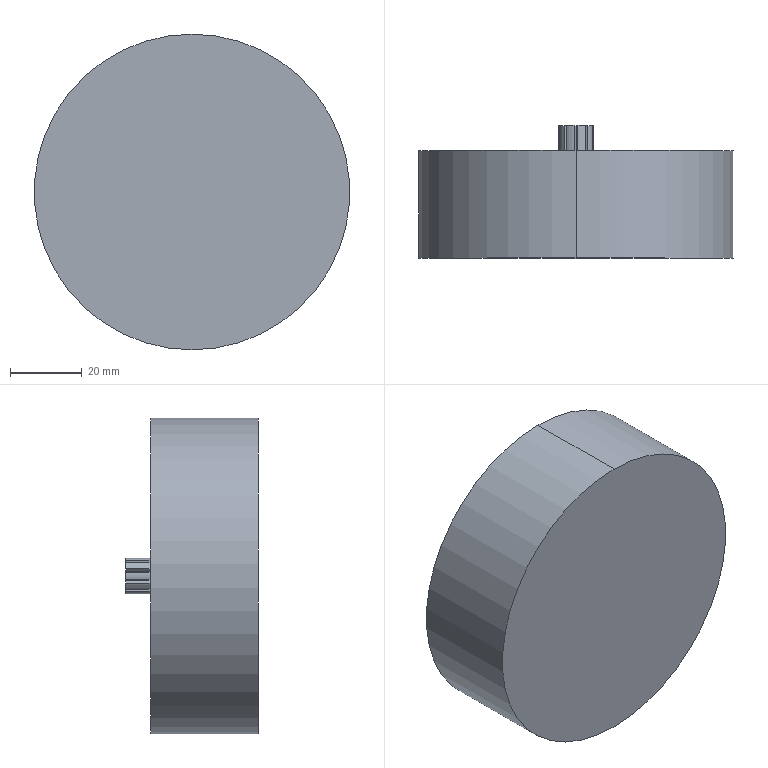Part | STEP file | Guide wheel mechanism revised.sldasm-Part-318 | 1 solid | 38 faces | box 88 x 37 x 88 mm | volume 180795 mm3 | plane 24 | cylinder 14 | commonest cylinder face diameters 10 x10 21 x2 88 x2
STEP:
#1=CARTESIAN_POINT('',(0.,30.,10.5));
#2=VERTEX_POINT('',#1);
#3=CARTESIAN_POINT('',(0.,30.,-10.5));
#4=VERTEX_POINT('',#3);
#5=CARTESIAN_POINT('',(0.,30.,0.));
#6=DIRECTION('',(0.,-1.,0.));
#7=DIRECTION('',(0.,0.,-1.));
#8=AXIS2_PLACEMENT_3D('',#5,#6,#7);
#9=CIRCLE('',#8,10.5);
#10=EDGE_CURVE('',#2,#4,#9,.T.);
#11=ORIENTED_EDGE('',*,*,#10,.F.);
#12=CARTESIAN_POINT('',(0.,22.,10.5));
#13=VERTEX_POINT('',#12);
#14=CARTESIAN_POINT('',(0.,0.,10.5));
#15=DIRECTION('',(0.,-1.,0.));
#16=VECTOR('',#15,1000.);
#17=LINE('',#14,#16);
#18=EDGE_CURVE('',#2,#13,#17,.T.);
#19=ORIENTED_EDGE('',*,*,#18,.T.);
#20=CARTESIAN_POINT('',(0.,22.,-10.5));
#21=VERTEX_POINT('',#20);
#22=CARTESIAN_POINT('',(0.,22.,0.));
#23=DIRECTION('',(0.,-1.,0.));
#24=DIRECTION('',(0.,0.,-1.));
#25=AXIS2_PLACEMENT_3D('',#22,#23,#24);
#26=CIRCLE('',#25,10.5);
#27=EDGE_CURVE('',#13,#21,#26,.T.);
#28=ORIENTED_EDGE('',*,*,#27,.T.);
#29=CARTESIAN_POINT('',(0.,0.,-10.5));
#30=DIRECTION('',(0.,-1.,0.));
#31=VECTOR('',#30,1000.);
#32=LINE('',#29,#31);
#33=EDGE_CURVE('',#4,#21,#32,.T.);
#34=ORIENTED_EDGE('',*,*,#33,.F.);
#35=EDGE_LOOP('',(#11,#19,#28,#34));
#36=FACE_OUTER_BOUND('',#35,.T.);
#37=CARTESIAN_POINT('',(0.,0.,0.));
#38=DIRECTION('',(0.,-1.,0.));
#39=DIRECTION('',(0.,0.,-1.));
#40=AXIS2_PLACEMENT_3D('',#37,#38,#39);
#41=CYLINDRICAL_SURFACE('',#40,10.5);
#42=ADVANCED_FACE('',(#36),#41,.F.);
#43=CARTESIAN_POINT('',(0.,30.,-44.));
#44=VERTEX_POINT('',#43);
#45=CARTESIAN_POINT('',(0.,30.,44.));
#46=VERTEX_POINT('',#45);
#47=CARTESIAN_POINT('',(0.,30.,0.));
#48=DIRECTION('',(0.,-1.,0.));
#49=DIRECTION('',(0.,0.,-1.));
#50=AXIS2_PLACEMENT_3D('',#47,#48,#49);
#51=CIRCLE('',#50,44.);
#52=EDGE_CURVE('',#44,#46,#51,.T.);
#53=ORIENTED_EDGE('',*,*,#52,.T.);
#54=CARTESIAN_POINT('',(0.,0.,44.));
#55=VERTEX_POINT('',#54);
#56=CARTESIAN_POINT('',(0.,0.,44.));
#57=DIRECTION('',(0.,-1.,0.));
#58=VECTOR('',#57,1000.);
#59=LINE('',#56,#58);
#60=EDGE_CURVE('',#46,#55,#59,.T.);
#61=ORIENTED_EDGE('',*,*,#60,.T.);
#62=CARTESIAN_POINT('',(0.,0.,-44.));
#63=VERTEX_POINT('',#62);
#64=CARTESIAN_POINT('',(0.,0.,0.));
#65=DIRECTION('',(0.,-1.,0.));
#66=DIRECTION('',(0.,0.,-1.));
#67=AXIS2_PLACEMENT_3D('',#64,#65,#66);
#68=CIRCLE('',#67,44.);
#69=EDGE_CURVE('',#63,#55,#68,.T.);
#70=ORIENTED_EDGE('',*,*,#69,.F.);
#71=CARTESIAN_POINT('',(0.,0.,-44.));
#72=DIRECTION('',(0.,-1.,0.));
#73=VECTOR('',#72,1000.);
#74=LINE('',#71,#73);
#75=EDGE_CURVE('',#44,#63,#74,.T.);
#76=ORIENTED_EDGE('',*,*,#75,.F.);
#77=EDGE_LOOP('',(#53,#61,#70,#76));
#78=FACE_OUTER_BOUND('',#77,.T.);
#79=CARTESIAN_POINT('',(0.,0.,0.));
#80=DIRECTION('',(0.,-1.,0.));
#81=DIRECTION('',(0.,0.,-1.));
#82=AXIS2_PLACEMENT_3D('',#79,#80,#81);
#83=CYLINDRICAL_SURFACE('',#82,44.);
#84=ADVANCED_FACE('',(#78),#83,.T.);
#85=CARTESIAN_POINT('',(-2.52,22.,-4.319));
#86=VERTEX_POINT('',#85);
#87=CARTESIAN_POINT('',(-2.52,37.,-4.319));
#88=VERTEX_POINT('',#87);
#89=CARTESIAN_POINT('',(-2.52,20.541,-4.319));
#90=DIRECTION('',(0.,1.,0.));
#91=VECTOR('',#90,1000.);
#92=LINE('',#89,#91);
#93=EDGE_CURVE('',#86,#88,#92,.T.);
#94=ORIENTED_EDGE('',*,*,#93,.T.);
#95=CARTESIAN_POINT('',(-0.5,37.,-4.975));
#96=VERTEX_POINT('',#95);
#97=CARTESIAN_POINT('',(0.,37.,0.));
#98=DIRECTION('',(0.,-1.,0.));
#99=DIRECTION('',(0.,0.,-1.));
#100=AXIS2_PLACEMENT_3D('',#97,#98,#99);
#101=CIRCLE('',#100,5.);
#102=EDGE_CURVE('',#88,#96,#101,.T.);
#103=ORIENTED_EDGE('',*,*,#102,.T.);
#104=CARTESIAN_POINT('',(-0.5,22.,-4.975));
#105=VERTEX_POINT('',#104);
#106=CARTESIAN_POINT('',(-0.5,20.586,-4.975));
#107=DIRECTION('',(0.,1.,0.));
#108=VECTOR('',#107,1000.);
#109=LINE('',#106,#108);
#110=EDGE_CURVE('',#105,#96,#109,.T.);
#111=ORIENTED_EDGE('',*,*,#110,.F.);
#112=CARTESIAN_POINT('',(0.,22.,0.));
#113=DIRECTION('',(0.,-1.,0.));
#114=DIRECTION('',(0.,0.,-1.));
#115=AXIS2_PLACEMENT_3D('',#112,#113,#114);
#116=CIRCLE('',#115,5.);
#117=EDGE_CURVE('',#86,#105,#116,.T.);
#118=ORIENTED_EDGE('',*,*,#117,.F.);
#119=EDGE_LOOP('',(#94,#103,#111,#118));
#120=FACE_OUTER_BOUND('',#119,.T.);
#121=CARTESIAN_POINT('',(0.,0.,0.));
#122=DIRECTION('',(0.,-1.,0.));
#123=DIRECTION('',(0.,0.,-1.));
#124=AXIS2_PLACEMENT_3D('',#121,#122,#123);
#125=CYLINDRICAL_SURFACE('',#124,5.);
#126=ADVANCED_FACE('',(#120),#125,.T.);
#127=CARTESIAN_POINT('',(-3.329,22.,-3.731));
#128=VERTEX_POINT('',#127);
#129=CARTESIAN_POINT('',(-3.329,37.,-3.731));
#130=VERTEX_POINT('',#129);
#131=CARTESIAN_POINT('',(-3.329,20.541,-3.731));
#132=DIRECTION('',(0.,1.,0.));
#133=VECTOR('',#132,1000.);
#134=LINE('',#131,#133);
#135=EDGE_CURVE('',#128,#130,#134,.T.);
#136=ORIENTED_EDGE('',*,*,#135,.F.);
#137=CARTESIAN_POINT('',(-4.577,22.,-2.013));
#138=VERTEX_POINT('',#137);
#139=CARTESIAN_POINT('',(0.,22.,0.));
#140=DIRECTION('',(0.,-1.,0.));
#141=DIRECTION('',(0.,0.,-1.));
#142=AXIS2_PLACEMENT_3D('',#139,#140,#141);
#143=CIRCLE('',#142,5.);
#144=EDGE_CURVE('',#138,#128,#143,.T.);
#145=ORIENTED_EDGE('',*,*,#144,.F.);
#146=CARTESIAN_POINT('',(-4.577,37.,-2.013));
#147=VERTEX_POINT('',#146);
#148=CARTESIAN_POINT('',(-4.577,20.56,-2.013));
#149=DIRECTION('',(0.,1.,0.));
#150=VECTOR('',#149,1000.);
#151=LINE('',#148,#150);
#152=EDGE_CURVE('',#138,#147,#151,.T.);
#153=ORIENTED_EDGE('',*,*,#152,.T.);
#154=CARTESIAN_POINT('',(0.,37.,0.));
#155=DIRECTION('',(0.,-1.,0.));
#156=DIRECTION('',(0.,0.,-1.));
#157=AXIS2_PLACEMENT_3D('',#154,#155,#156);
#158=CIRCLE('',#157,5.);
#159=EDGE_CURVE('',#147,#130,#158,.T.);
#160=ORIENTED_EDGE('',*,*,#159,.T.);
#161=EDGE_LOOP('',(#136,#145,#153,#160));
#162=FACE_OUTER_BOUND('',#161,.T.);
#163=CARTESIAN_POINT('',(0.,0.,0.));
#164=DIRECTION('',(0.,-1.,0.));
#165=DIRECTION('',(0.,0.,-1.));
#166=AXIS2_PLACEMENT_3D('',#163,#164,#165);
#167=CYLINDRICAL_SURFACE('',#166,5.);
#168=ADVANCED_FACE('',(#162),#167,.T.);
#169=CARTESIAN_POINT('',(-4.886,22.,-1.062));
#170=VERTEX_POINT('',#169);
#171=CARTESIAN_POINT('',(-4.886,37.,-1.062));
#172=VERTEX_POINT('',#171);
#173=CARTESIAN_POINT('',(-4.886,20.56,-1.062));
#174=DIRECTION('',(0.,1.,0.));
#175=VECTOR('',#174,1000.);
#176=LINE('',#173,#175);
#177=EDGE_CURVE('',#170,#172,#176,.T.);
#178=ORIENTED_EDGE('',*,*,#177,.F.);
#179=CARTESIAN_POINT('',(-4.886,22.,1.062));
#180=VERTEX_POINT('',#179);
#181=CARTESIAN_POINT('',(0.,22.,0.));
#182=DIRECTION('',(0.,-1.,0.));
#183=DIRECTION('',(0.,0.,-1.));
#184=AXIS2_PLACEMENT_3D('',#181,#182,#183);
#185=CIRCLE('',#184,5.);
#186=EDGE_CURVE('',#180,#170,#185,.T.);
#187=ORIENTED_EDGE('',*,*,#186,.F.);
#188=CARTESIAN_POINT('',(-4.886,37.,1.062));
#189=VERTEX_POINT('',#188);
#190=CARTESIAN_POINT('',(-4.886,20.56,1.062));
#191=DIRECTION('',(0.,1.,0.));
#192=VECTOR('',#191,1000.);
#193=LINE('',#190,#192);
#194=EDGE_CURVE('',#180,#189,#193,.T.);
#195=ORIENTED_EDGE('',*,*,#194,.T.);
#196=CARTESIAN_POINT('',(0.,37.,0.));
#197=DIRECTION('',(0.,-1.,0.));
#198=DIRECTION('',(0.,0.,-1.));
#199=AXIS2_PLACEMENT_3D('',#196,#197,#198);
#200=CIRCLE('',#199,5.);
#201=EDGE_CURVE('',#189,#172,#200,.T.);
#202=ORIENTED_EDGE('',*,*,#201,.T.);
#203=EDGE_LOOP('',(#178,#187,#195,#202));
#204=FACE_OUTER_BOUND('',#203,.T.);
#205=CARTESIAN_POINT('',(0.,0.,0.));
#206=DIRECTION('',(0.,-1.,0.));
#207=DIRECTION('',(0.,0.,-1.));
#208=AXIS2_PLACEMENT_3D('',#205,#206,#207);
#209=CYLINDRICAL_SURFACE('',#208,5.);
#210=ADVANCED_FACE('',(#204),#209,.T.);
#211=CARTESIAN_POINT('',(-4.577,22.,2.013));
#212=VERTEX_POINT('',#211);
#213=CARTESIAN_POINT('',(-4.577,37.,2.013));
#214=VERTEX_POINT('',#213);
#215=CARTESIAN_POINT('',(-4.577,20.56,2.013));
#216=DIRECTION('',(0.,1.,0.));
#217=VECTOR('',#216,1000.);
#218=LINE('',#215,#217);
#219=EDGE_CURVE('',#212,#214,#218,.T.);
#220=ORIENTED_EDGE('',*,*,#219,.F.);
#221=CARTESIAN_POINT('',(-3.329,22.,3.731));
#222=VERTEX_POINT('',#221);
#223=CARTESIAN_POINT('',(0.,22.,0.));
#224=DIRECTION('',(0.,-1.,0.));
#225=DIRECTION('',(0.,0.,-1.));
#226=AXIS2_PLACEMENT_3D('',#223,#224,#225);
#227=CIRCLE('',#226,5.);
#228=EDGE_CURVE('',#222,#212,#227,.T.);
#229=ORIENTED_EDGE('',*,*,#228,.F.);
#230=CARTESIAN_POINT('',(-3.329,37.,3.731));
#231=VERTEX_POINT('',#230);
#232=CARTESIAN_POINT('',(-3.329,20.541,3.731));
#233=DIRECTION('',(0.,1.,0.));
#234=VECTOR('',#233,1000.);
#235=LINE('',#232,#234);
#236=EDGE_CURVE('',#222,#231,#235,.T.);
#237=ORIENTED_EDGE('',*,*,#236,.T.);
#238=CARTESIAN_POINT('',(0.,37.,0.));
#239=DIRECTION('',(0.,-1.,0.));
#240=DIRECTION('',(0.,0.,-1.));
#241=AXIS2_PLACEMENT_3D('',#238,#239,#240);
#242=CIRCLE('',#241,5.);
#243=EDGE_CURVE('',#231,#214,#242,.T.);
#244=ORIENTED_EDGE('',*,*,#243,.T.);
#245=EDGE_LOOP('',(#220,#229,#237,#244));
#246=FACE_OUTER_BOUND('',#245,.T.);
#247=CARTESIAN_POINT('',(0.,0.,0.));
#248=DIRECTION('',(0.,-1.,0.));
#249=DIRECTION('',(0.,0.,-1.));
#250=AXIS2_PLACEMENT_3D('',#247,#248,#249);
#251=CYLINDRICAL_SURFACE('',#250,5.);
#252=ADVANCED_FACE('',(#246),#251,.T.);
#253=CARTESIAN_POINT('',(-2.52,22.,4.319));
#254=VERTEX_POINT('',#253);
#255=CARTESIAN_POINT('',(-2.52,37.,4.319));
#256=VERTEX_POINT('',#255);
#257=CARTESIAN_POINT('',(-2.52,20.541,4.319));
#258=DIRECTION('',(0.,1.,0.));
#259=VECTOR('',#258,1000.);
#260=LINE('',#257,#259);
#261=EDGE_CURVE('',#254,#256,#260,.T.);
#262=ORIENTED_EDGE('',*,*,#261,.F.);
#263=CARTESIAN_POINT('',(-0.5,22.,4.975));
#264=VERTEX_POINT('',#263);
#265=CARTESIAN_POINT('',(0.,22.,0.));
#266=DIRECTION('',(0.,-1.,0.));
#267=DIRECTION('',(0.,0.,-1.));
#268=AXIS2_PLACEMENT_3D('',#265,#266,#267);
#269=CIRCLE('',#268,5.);
#270=EDGE_CURVE('',#264,#254,#269,.T.);
#271=ORIENTED_EDGE('',*,*,#270,.F.);
#272=CARTESIAN_POINT('',(-0.5,37.,4.975));
#273=VERTEX_POINT('',#272);
#274=CARTESIAN_POINT('',(-0.5,20.586,4.975));
#275=DIRECTION('',(0.,1.,0.));
#276=VECTOR('',#275,1000.);
#277=LINE('',#274,#276);
#278=EDGE_CURVE('',#264,#273,#277,.T.);
#279=ORIENTED_EDGE('',*,*,#278,.T.);
#280=CARTESIAN_POINT('',(0.,37.,0.));
#281=DIRECTION('',(0.,-1.,0.));
#282=DIRECTION('',(0.,0.,-1.));
#283=AXIS2_PLACEMENT_3D('',#280,#281,#282);
#284=CIRCLE('',#283,5.);
#285=EDGE_CURVE('',#273,#256,#284,.T.);
#286=ORIENTED_EDGE('',*,*,#285,.T.);
#287=EDGE_LOOP('',(#262,#271,#279,#286));
#288=FACE_OUTER_BOUND('',#287,.T.);
#289=CARTESIAN_POINT('',(0.,0.,0.));
#290=DIRECTION('',(0.,-1.,0.));
#291=DIRECTION('',(0.,0.,-1.));
#292=AXIS2_PLACEMENT_3D('',#289,#290,#291);
#293=CYLINDRICAL_SURFACE('',#292,5.);
#294=ADVANCED_FACE('',(#288),#293,.T.);
#295=CARTESIAN_POINT('',(0.5,22.,4.975));
#296=VERTEX_POINT('',#295);
#297=CARTESIAN_POINT('',(0.5,37.,4.975));
#298=VERTEX_POINT('',#297);
#299=CARTESIAN_POINT('',(0.5,20.586,4.975));
#300=DIRECTION('',(0.,1.,0.));
#301=VECTOR('',#300,1000.);
#302=LINE('',#299,#301);
#303=EDGE_CURVE('',#296,#298,#302,.T.);
#304=ORIENTED_EDGE('',*,*,#303,.F.);
#305=CARTESIAN_POINT('',(2.52,22.,4.319));
#306=VERTEX_POINT('',#305);
#307=CARTESIAN_POINT('',(0.,22.,0.));
#308=DIRECTION('',(0.,-1.,0.));
#309=DIRECTION('',(0.,0.,-1.));
#310=AXIS2_PLACEMENT_3D('',#307,#308,#309);
#311=CIRCLE('',#310,5.);
#312=EDGE_CURVE('',#306,#296,#311,.T.);
#313=ORIENTED_EDGE('',*,*,#312,.F.);
#314=CARTESIAN_POINT('',(2.52,37.,4.319));
#315=VERTEX_POINT('',#314);
#316=CARTESIAN_POINT('',(2.52,20.541,4.319));
#317=DIRECTION('',(0.,1.,0.));
#318=VECTOR('',#317,1000.);
#319=LINE('',#316,#318);
#320=EDGE_CURVE('',#306,#315,#319,.T.);
#321=ORIENTED_EDGE('',*,*,#320,.T.);
#322=CARTESIAN_POINT('',(0.,37.,0.));
#323=DIRECTION('',(0.,-1.,0.));
#324=DIRECTION('',(0.,0.,-1.));
#325=AXIS2_PLACEMENT_3D('',#322,#323,#324);
#326=CIRCLE('',#325,5.);
#327=EDGE_CURVE('',#315,#298,#326,.T.);
#328=ORIENTED_EDGE('',*,*,#327,.T.);
#329=EDGE_LOOP('',(#304,#313,#321,#328));
#330=FACE_OUTER_BOUND('',#329,.T.);
#331=CARTESIAN_POINT('',(0.,0.,0.));
#332=DIRECTION('',(0.,-1.,0.));
#333=DIRECTION('',(0.,0.,-1.));
#334=AXIS2_PLACEMENT_3D('',#331,#332,#333);
#335=CYLINDRICAL_SURFACE('',#334,5.);
#336=ADVANCED_FACE('',(#330),#335,.T.);
#337=CARTESIAN_POINT('',(3.329,22.,3.731));
#338=VERTEX_POINT('',#337);
#339=CARTESIAN_POINT('',(3.329,37.,3.731));
#340=VERTEX_POINT('',#339);
#341=CARTESIAN_POINT('',(3.329,20.541,3.731));
#342=DIRECTION('',(0.,1.,0.));
#343=VECTOR('',#342,1000.);
#344=LINE('',#341,#343);
#345=EDGE_CURVE('',#338,#340,#344,.T.);
#346=ORIENTED_EDGE('',*,*,#345,.F.);
#347=CARTESIAN_POINT('',(4.577,22.,2.013));
#348=VERTEX_POINT('',#347);
#349=CARTESIAN_POINT('',(0.,22.,0.));
#350=DIRECTION('',(0.,-1.,0.));
#351=DIRECTION('',(0.,0.,-1.));
#352=AXIS2_PLACEMENT_3D('',#349,#350,#351);
#353=CIRCLE('',#352,5.);
#354=EDGE_CURVE('',#348,#338,#353,.T.);
#355=ORIENTED_EDGE('',*,*,#354,.F.);
#356=CARTESIAN_POINT('',(4.577,37.,2.013));
#357=VERTEX_POINT('',#356);
#358=CARTESIAN_POINT('',(4.577,20.56,2.013));
#359=DIRECTION('',(0.,1.,0.));
#360=VECTOR('',#359,1000.);
#361=LINE('',#358,#360);
#362=EDGE_CURVE('',#348,#357,#361,.T.);
#363=ORIENTED_EDGE('',*,*,#362,.T.);
#364=CARTESIAN_POINT('',(0.,37.,0.));
#365=DIRECTION('',(0.,-1.,0.));
#366=DIRECTION('',(0.,0.,-1.));
#367=AXIS2_PLACEMENT_3D('',#364,#365,#366);
#368=CIRCLE('',#367,5.);
#369=EDGE_CURVE('',#357,#340,#368,.T.);
#370=ORIENTED_EDGE('',*,*,#369,.T.);
#371=EDGE_LOOP('',(#346,#355,#363,#370));
#372=FACE_OUTER_BOUND('',#371,.T.);
#373=CARTESIAN_POINT('',(0.,0.,0.));
#374=DIRECTION('',(0.,-1.,0.));
#375=DIRECTION('',(0.,0.,-1.));
#376=AXIS2_PLACEMENT_3D('',#373,#374,#375);
#377=CYLINDRICAL_SURFACE('',#376,5.);
#378=ADVANCED_FACE('',(#372),#377,.T.);
#379=CARTESIAN_POINT('',(4.886,22.,1.062));
#380=VERTEX_POINT('',#379);
#381=CARTESIAN_POINT('',(4.886,37.,1.062));
#382=VERTEX_POINT('',#381);
#383=CARTESIAN_POINT('',(4.886,20.56,1.062));
#384=DIRECTION('',(0.,1.,0.));
#385=VECTOR('',#384,1000.);
#386=LINE('',#383,#385);
#387=EDGE_CURVE('',#380,#382,#386,.T.);
#388=ORIENTED_EDGE('',*,*,#387,.F.);
#389=CARTESIAN_POINT('',(4.886,22.,-1.062));
#390=VERTEX_POINT('',#389);
#391=CARTESIAN_POINT('',(0.,22.,0.));
#392=DIRECTION('',(0.,-1.,0.));
#393=DIRECTION('',(0.,0.,-1.));
#394=AXIS2_PLACEMENT_3D('',#391,#392,#393);
#395=CIRCLE('',#394,5.);
#396=EDGE_CURVE('',#390,#380,#395,.T.);
#397=ORIENTED_EDGE('',*,*,#396,.F.);
#398=CARTESIAN_POINT('',(4.886,37.,-1.062));
#399=VERTEX_POINT('',#398);
#400=CARTESIAN_POINT('',(4.886,20.56,-1.062));
#401=DIRECTION('',(0.,1.,0.));
#402=VECTOR('',#401,1000.);
#403=LINE('',#400,#402);
#404=EDGE_CURVE('',#390,#399,#403,.T.);
#405=ORIENTED_EDGE('',*,*,#404,.T.);
#406=CARTESIAN_POINT('',(0.,37.,0.));
#407=DIRECTION('',(0.,-1.,0.));
#408=DIRECTION('',(0.,0.,-1.));
#409=AXIS2_PLACEMENT_3D('',#406,#407,#408);
#410=CIRCLE('',#409,5.);
#411=EDGE_CURVE('',#399,#382,#410,.T.);
#412=ORIENTED_EDGE('',*,*,#411,.T.);
#413=EDGE_LOOP('',(#388,#397,#405,#412));
#414=FACE_OUTER_BOUND('',#413,.T.);
#415=CARTESIAN_POINT('',(0.,0.,0.));
#416=DIRECTION('',(0.,-1.,0.));
#417=DIRECTION('',(0.,0.,-1.));
#418=AXIS2_PLACEMENT_3D('',#415,#416,#417);
#419=CYLINDRICAL_SURFACE('',#418,5.);
#420=ADVANCED_FACE('',(#414),#419,.T.);
#421=CARTESIAN_POINT('',(4.577,22.,-2.013));
#422=VERTEX_POINT('',#421);
#423=CARTESIAN_POINT('',(4.577,37.,-2.013));
#424=VERTEX_POINT('',#423);
#425=CARTESIAN_POINT('',(4.577,20.56,-2.013));
#426=DIRECTION('',(0.,1.,0.));
#427=VECTOR('',#426,1000.);
#428=LINE('',#425,#427);
#429=EDGE_CURVE('',#422,#424,#428,.T.);
#430=ORIENTED_EDGE('',*,*,#429,.F.);
#431=CARTESIAN_POINT('',(3.329,22.,-3.731));
#432=VERTEX_POINT('',#431);
#433=CARTESIAN_POINT('',(0.,22.,0.));
#434=DIRECTION('',(0.,-1.,0.));
#435=DIRECTION('',(0.,0.,-1.));
#436=AXIS2_PLACEMENT_3D('',#433,#434,#435);
#437=CIRCLE('',#436,5.);
#438=EDGE_CURVE('',#432,#422,#437,.T.);
#439=ORIENTED_EDGE('',*,*,#438,.F.);
#440=CARTESIAN_POINT('',(3.329,37.,-3.731));
#441=VERTEX_POINT('',#440);
#442=CARTESIAN_POINT('',(3.329,20.541,-3.731));
#443=DIRECTION('',(0.,1.,0.));
#444=VECTOR('',#443,1000.);
#445=LINE('',#442,#444);
#446=EDGE_CURVE('',#432,#441,#445,.T.);
#447=ORIENTED_EDGE('',*,*,#446,.T.);
#448=CARTESIAN_POINT('',(0.,37.,0.));
#449=DIRECTION('',(0.,-1.,0.));
#450=DIRECTION('',(0.,0.,-1.));
#451=AXIS2_PLACEMENT_3D('',#448,#449,#450);
#452=CIRCLE('',#451,5.);
#453=EDGE_CURVE('',#441,#424,#452,.T.);
#454=ORIENTED_EDGE('',*,*,#453,.T.);
#455=EDGE_LOOP('',(#430,#439,#447,#454));
#456=FACE_OUTER_BOUND('',#455,.T.);
#457=CARTESIAN_POINT('',(0.,0.,0.));
#458=DIRECTION('',(0.,-1.,0.));
#459=DIRECTION('',(0.,0.,-1.));
#460=AXIS2_PLACEMENT_3D('',#457,#458,#459);
#461=CYLINDRICAL_SURFACE('',#460,5.);
#462=ADVANCED_FACE('',(#456),#461,.T.);
#463=ORIENTED_EDGE('',*,*,#69,.T.);
#464=CARTESIAN_POINT('',(0.,0.,0.));
#465=DIRECTION('',(0.,-1.,0.));
#466=DIRECTION('',(0.,0.,-1.));
#467=AXIS2_PLACEMENT_3D('',#464,#465,#466);
#468=CIRCLE('',#467,44.);
#469=EDGE_CURVE('',#55,#63,#468,.T.);
#470=ORIENTED_EDGE('',*,*,#469,.T.);
#471=EDGE_LOOP('',(#463,#470));
#472=FACE_OUTER_BOUND('',#471,.T.);
#473=CARTESIAN_POINT('',(0.,0.,0.));
#474=DIRECTION('',(0.,-1.,0.));
#475=DIRECTION('',(0.,0.,-1.));
#476=AXIS2_PLACEMENT_3D('',#473,#474,#475);
#477=PLANE('',#476);
#478=ADVANCED_FACE('',(#472),#477,.T.);
#479=ORIENTED_EDGE('',*,*,#60,.F.);
#480=CARTESIAN_POINT('',(0.,30.,0.));
#481=DIRECTION('',(0.,-1.,0.));
#482=DIRECTION('',(0.,0.,-1.));
#483=AXIS2_PLACEMENT_3D('',#480,#481,#482);
#484=CIRCLE('',#483,44.);
#485=EDGE_CURVE('',#46,#44,#484,.T.);
#486=ORIENTED_EDGE('',*,*,#485,.T.);
#487=ORIENTED_EDGE('',*,*,#75,.T.);
#488=ORIENTED_EDGE('',*,*,#469,.F.);
#489=EDGE_LOOP('',(#479,#486,#487,#488));
#490=FACE_OUTER_BOUND('',#489,.T.);
#491=CARTESIAN_POINT('',(0.,0.,0.));
#492=DIRECTION('',(0.,-1.,0.));
#493=DIRECTION('',(0.,0.,-1.));
#494=AXIS2_PLACEMENT_3D('',#491,#492,#493);
#495=CYLINDRICAL_SURFACE('',#494,44.);
#496=ADVANCED_FACE('',(#490),#495,.T.);
#497=CARTESIAN_POINT('',(0.,30.,0.));
#498=DIRECTION('',(0.,-1.,0.));
#499=DIRECTION('',(0.,0.,-1.));
#500=AXIS2_PLACEMENT_3D('',#497,#498,#499);
#501=CIRCLE('',#500,10.5);
#502=EDGE_CURVE('',#4,#2,#501,.T.);
#503=ORIENTED_EDGE('',*,*,#502,.T.);
#504=ORIENTED_EDGE('',*,*,#10,.T.);
#505=EDGE_LOOP('',(#503,#504));
#506=FACE_BOUND('',#505,.T.);
#507=ORIENTED_EDGE('',*,*,#52,.F.);
#508=ORIENTED_EDGE('',*,*,#485,.F.);
#509=EDGE_LOOP('',(#507,#508));
#510=FACE_OUTER_BOUND('',#509,.T.);
#511=CARTESIAN_POINT('',(44.,30.,0.));
#512=DIRECTION('',(0.,1.,0.));
#513=DIRECTION('',(0.,0.,1.));
#514=AXIS2_PLACEMENT_3D('',#511,#512,#513);
#515=PLANE('',#514);
#516=ADVANCED_FACE('',(#506,#510),#515,.T.);
#517=ORIENTED_EDGE('',*,*,#18,.F.);
#518=ORIENTED_EDGE('',*,*,#502,.F.);
#519=ORIENTED_EDGE('',*,*,#33,.T.);
#520=CARTESIAN_POINT('',(0.,22.,0.));
#521=DIRECTION('',(0.,-1.,0.));
#522=DIRECTION('',(0.,0.,-1.));
#523=AXIS2_PLACEMENT_3D('',#520,#521,#522);
#524=CIRCLE('',#523,10.5);
#525=EDGE_CURVE('',#21,#13,#524,.T.);
#526=ORIENTED_EDGE('',*,*,#525,.T.);
#527=EDGE_LOOP('',(#517,#518,#519,#526));
#528=FACE_OUTER_BOUND('',#527,.T.);
#529=CARTESIAN_POINT('',(0.,0.,0.));
#530=DIRECTION('',(0.,-1.,0.));
#531=DIRECTION('',(0.,0.,-1.));
#532=AXIS2_PLACEMENT_3D('',#529,#530,#531);
#533=CYLINDRICAL_SURFACE('',#532,10.5);
#534=ADVANCED_FACE('',(#528),#533,.F.);
#535=CARTESIAN_POINT('',(0.5,22.,-4.975));
#536=VERTEX_POINT('',#535);
#537=CARTESIAN_POINT('',(2.52,22.,-4.319));
#538=VERTEX_POINT('',#537);
#539=CARTESIAN_POINT('',(0.,22.,0.));
#540=DIRECTION('',(0.,-1.,0.));
#541=DIRECTION('',(0.,0.,-1.));
#542=AXIS2_PLACEMENT_3D('',#539,#540,#541);
#543=CIRCLE('',#542,5.);
#544=EDGE_CURVE('',#536,#538,#543,.T.);
#545=ORIENTED_EDGE('',*,*,#544,.T.);
#546=CARTESIAN_POINT('',(2.351,22.,-3.236));
#547=VERTEX_POINT('',#546);
#548=CARTESIAN_POINT('',(2.52,22.,-4.319));
#549=DIRECTION('',(0.1538,0.,-0.9881));
#550=VECTOR('',#549,1000.);
#551=LINE('',#548,#550);
#552=EDGE_CURVE('',#547,#538,#551,.T.);
#553=ORIENTED_EDGE('',*,*,#552,.F.);
#554=CARTESIAN_POINT('',(2.351,22.,-3.236));
#555=DIRECTION('',(-0.8922,0.,0.4516));
#556=VECTOR('',#555,1000.);
#557=LINE('',#554,#556);
#558=EDGE_CURVE('',#432,#547,#557,.T.);
#559=ORIENTED_EDGE('',*,*,#558,.F.);
#560=ORIENTED_EDGE('',*,*,#438,.T.);
#561=CARTESIAN_POINT('',(3.804,22.,-1.236));
#562=VERTEX_POINT('',#561);
#563=CARTESIAN_POINT('',(4.577,22.,-2.013));
#564=DIRECTION('',(0.7052,0.,-0.709));
#565=VECTOR('',#564,1000.);
#566=LINE('',#563,#565);
#567=EDGE_CURVE('',#562,#422,#566,.T.);
#568=ORIENTED_EDGE('',*,*,#567,.F.);
#569=CARTESIAN_POINT('',(3.804,22.,-1.236));
#570=DIRECTION('',(-0.9873,0.,-0.159));
#571=VECTOR('',#570,1000.);
#572=LINE('',#569,#571);
#573=EDGE_CURVE('',#390,#562,#572,.T.);
#574=ORIENTED_EDGE('',*,*,#573,.F.);
#575=ORIENTED_EDGE('',*,*,#396,.T.);
#576=CARTESIAN_POINT('',(3.804,22.,1.236));
#577=VERTEX_POINT('',#576);
#578=CARTESIAN_POINT('',(4.886,22.,1.062));
#579=DIRECTION('',(0.9873,0.,-0.159));
#580=VECTOR('',#579,1000.);
#581=LINE('',#578,#580);
#582=EDGE_CURVE('',#577,#380,#581,.T.);
#583=ORIENTED_EDGE('',*,*,#582,.F.);
#584=CARTESIAN_POINT('',(3.804,22.,1.236));
#585=DIRECTION('',(-0.7052,0.,-0.709));
#586=VECTOR('',#585,1000.);
#587=LINE('',#584,#586);
#588=EDGE_CURVE('',#348,#577,#587,.T.);
#589=ORIENTED_EDGE('',*,*,#588,.F.);
#590=ORIENTED_EDGE('',*,*,#354,.T.);
#591=CARTESIAN_POINT('',(2.351,22.,3.236));
#592=VERTEX_POINT('',#591);
#593=CARTESIAN_POINT('',(3.329,22.,3.731));
#594=DIRECTION('',(0.8922,0.,0.4516));
#595=VECTOR('',#594,1000.);
#596=LINE('',#593,#595);
#597=EDGE_CURVE('',#592,#338,#596,.T.);
#598=ORIENTED_EDGE('',*,*,#597,.F.);
#599=CARTESIAN_POINT('',(2.351,22.,3.236));
#600=DIRECTION('',(-0.1538,0.,-0.9881));
#601=VECTOR('',#600,1000.);
#602=LINE('',#599,#601);
#603=EDGE_CURVE('',#306,#592,#602,.T.);
#604=ORIENTED_EDGE('',*,*,#603,.F.);
#605=ORIENTED_EDGE('',*,*,#312,.T.);
#606=CARTESIAN_POINT('',(0.,22.,4.));
#607=VERTEX_POINT('',#606);
#608=CARTESIAN_POINT('',(0.5,22.,4.975));
#609=DIRECTION('',(0.4563,0.,0.8898));
#610=VECTOR('',#609,1000.);
#611=LINE('',#608,#610);
#612=EDGE_CURVE('',#607,#296,#611,.T.);
#613=ORIENTED_EDGE('',*,*,#612,.F.);
#614=CARTESIAN_POINT('',(0.,22.,4.));
#615=DIRECTION('',(0.4563,0.,-0.8898));
#616=VECTOR('',#615,1000.);
#617=LINE('',#614,#616);
#618=EDGE_CURVE('',#264,#607,#617,.T.);
#619=ORIENTED_EDGE('',*,*,#618,.F.);
#620=ORIENTED_EDGE('',*,*,#270,.T.);
#621=CARTESIAN_POINT('',(-2.351,22.,3.236));
#622=VERTEX_POINT('',#621);
#623=CARTESIAN_POINT('',(-2.52,22.,4.319));
#624=DIRECTION('',(-0.1538,0.,0.9881));
#625=VECTOR('',#624,1000.);
#626=LINE('',#623,#625);
#627=EDGE_CURVE('',#622,#254,#626,.T.);
#628=ORIENTED_EDGE('',*,*,#627,.F.);
#629=CARTESIAN_POINT('',(-2.351,22.,3.236));
#630=DIRECTION('',(0.8922,0.,-0.4516));
#631=VECTOR('',#630,1000.);
#632=LINE('',#629,#631);
#633=EDGE_CURVE('',#222,#622,#632,.T.);
#634=ORIENTED_EDGE('',*,*,#633,.F.);
#635=ORIENTED_EDGE('',*,*,#228,.T.);
#636=CARTESIAN_POINT('',(-3.804,22.,1.236));
#637=VERTEX_POINT('',#636);
#638=CARTESIAN_POINT('',(-4.577,22.,2.013));
#639=DIRECTION('',(-0.7052,0.,0.709));
#640=VECTOR('',#639,1000.);
#641=LINE('',#638,#640);
#642=EDGE_CURVE('',#637,#212,#641,.T.);
#643=ORIENTED_EDGE('',*,*,#642,.F.);
#644=CARTESIAN_POINT('',(-3.804,22.,1.236));
#645=DIRECTION('',(0.9873,0.,0.159));
#646=VECTOR('',#645,1000.);
#647=LINE('',#644,#646);
#648=EDGE_CURVE('',#180,#637,#647,.T.);
#649=ORIENTED_EDGE('',*,*,#648,.F.);
#650=ORIENTED_EDGE('',*,*,#186,.T.);
#651=CARTESIAN_POINT('',(-3.804,22.,-1.236));
#652=VERTEX_POINT('',#651);
#653=CARTESIAN_POINT('',(-4.886,22.,-1.062));
#654=DIRECTION('',(-0.9873,0.,0.159));
#655=VECTOR('',#654,1000.);
#656=LINE('',#653,#655);
#657=EDGE_CURVE('',#652,#170,#656,.T.);
#658=ORIENTED_EDGE('',*,*,#657,.F.);
#659=CARTESIAN_POINT('',(-3.804,22.,-1.236));
#660=DIRECTION('',(0.7052,0.,0.709));
#661=VECTOR('',#660,1000.);
#662=LINE('',#659,#661);
#663=EDGE_CURVE('',#138,#652,#662,.T.);
#664=ORIENTED_EDGE('',*,*,#663,.F.);
#665=ORIENTED_EDGE('',*,*,#144,.T.);
#666=CARTESIAN_POINT('',(-2.351,22.,-3.236));
#667=VERTEX_POINT('',#666);
#668=CARTESIAN_POINT('',(-3.329,22.,-3.731));
#669=DIRECTION('',(-0.8922,0.,-0.4516));
#670=VECTOR('',#669,1000.);
#671=LINE('',#668,#670);
#672=EDGE_CURVE('',#667,#128,#671,.T.);
#673=ORIENTED_EDGE('',*,*,#672,.F.);
#674=CARTESIAN_POINT('',(-2.351,22.,-3.236));
#675=DIRECTION('',(0.1538,0.,0.9881));
#676=VECTOR('',#675,1000.);
#677=LINE('',#674,#676);
#678=EDGE_CURVE('',#86,#667,#677,.T.);
#679=ORIENTED_EDGE('',*,*,#678,.F.);
#680=ORIENTED_EDGE('',*,*,#117,.T.);
#681=CARTESIAN_POINT('',(0.,22.,-4.));
#682=VERTEX_POINT('',#681);
#683=CARTESIAN_POINT('',(-0.5,22.,-4.975));
#684=DIRECTION('',(-0.4563,0.,-0.8898));
#685=VECTOR('',#684,1000.);
#686=LINE('',#683,#685);
#687=EDGE_CURVE('',#682,#105,#686,.T.);
#688=ORIENTED_EDGE('',*,*,#687,.F.);
#689=CARTESIAN_POINT('',(0.,22.,-4.));
#690=DIRECTION('',(-0.4563,0.,0.8898));
#691=VECTOR('',#690,1000.);
#692=LINE('',#689,#691);
#693=EDGE_CURVE('',#536,#682,#692,.T.);
#694=ORIENTED_EDGE('',*,*,#693,.F.);
#695=EDGE_LOOP('',(#545,#553,#559,#560,#568,#574,#575,#583,#589,#590,#598,#604,#605,#613,#619,#620,#628,#634,#635,#643,#649,#650,#658,#664,#665,#673,#679,#680,#688,#694));
#696=FACE_BOUND('',#695,.T.);
#697=ORIENTED_EDGE('',*,*,#525,.F.);
#698=ORIENTED_EDGE('',*,*,#27,.F.);
#699=EDGE_LOOP('',(#697,#698));
#700=FACE_OUTER_BOUND('',#699,.T.);
#701=CARTESIAN_POINT('',(10.5,22.,0.));
#702=DIRECTION('',(0.,1.,0.));
#703=DIRECTION('',(0.,0.,1.));
#704=AXIS2_PLACEMENT_3D('',#701,#702,#703);
#705=PLANE('',#704);
#706=ADVANCED_FACE('',(#696,#700),#705,.T.);
#707=CARTESIAN_POINT('',(2.52,37.,-4.319));
#708=VERTEX_POINT('',#707);
#709=CARTESIAN_POINT('',(2.52,20.541,-4.319));
#710=DIRECTION('',(0.,1.,0.));
#711=VECTOR('',#710,1000.);
#712=LINE('',#709,#711);
#713=EDGE_CURVE('',#538,#708,#712,.T.);
#714=ORIENTED_EDGE('',*,*,#713,.F.);
#715=ORIENTED_EDGE('',*,*,#544,.F.);
#716=CARTESIAN_POINT('',(0.5,37.,-4.975));
#717=VERTEX_POINT('',#716);
#718=CARTESIAN_POINT('',(0.5,20.586,-4.975));
#719=DIRECTION('',(0.,1.,0.));
#720=VECTOR('',#719,1000.);
#721=LINE('',#718,#720);
#722=EDGE_CURVE('',#536,#717,#721,.T.);
#723=ORIENTED_EDGE('',*,*,#722,.T.);
#724=CARTESIAN_POINT('',(0.,37.,0.));
#725=DIRECTION('',(0.,-1.,0.));
#726=DIRECTION('',(0.,0.,-1.));
#727=AXIS2_PLACEMENT_3D('',#724,#725,#726);
#728=CIRCLE('',#727,5.);
#729=EDGE_CURVE('',#717,#708,#728,.T.);
#730=ORIENTED_EDGE('',*,*,#729,.T.);
#731=EDGE_LOOP('',(#714,#715,#723,#730));
#732=FACE_OUTER_BOUND('',#731,.T.);
#733=CARTESIAN_POINT('',(0.,0.,0.));
#734=DIRECTION('',(0.,-1.,0.));
#735=DIRECTION('',(0.,0.,-1.));
#736=AXIS2_PLACEMENT_3D('',#733,#734,#735);
#737=CYLINDRICAL_SURFACE('',#736,5.);
#738=ADVANCED_FACE('',(#732),#737,.T.);
#739=CARTESIAN_POINT('',(-2.351,37.,-3.236));
#740=VERTEX_POINT('',#739);
#741=CARTESIAN_POINT('',(-2.351,37.,-3.236));
#742=DIRECTION('',(-0.1538,0.,-0.9881));
#743=VECTOR('',#742,1000.);
#744=LINE('',#741,#743);
#745=EDGE_CURVE('',#740,#88,#744,.T.);
#746=ORIENTED_EDGE('',*,*,#745,.F.);
#747=CARTESIAN_POINT('',(-3.329,37.,-3.731));
#748=DIRECTION('',(0.8922,0.,0.4516));
#749=VECTOR('',#748,1000.);
#750=LINE('',#747,#749);
#751=EDGE_CURVE('',#130,#740,#750,.T.);
#752=ORIENTED_EDGE('',*,*,#751,.F.);
#753=ORIENTED_EDGE('',*,*,#159,.F.);
#754=CARTESIAN_POINT('',(-3.804,37.,-1.236));
#755=VERTEX_POINT('',#754);
#756=CARTESIAN_POINT('',(-3.804,37.,-1.236));
#757=DIRECTION('',(-0.7052,0.,-0.709));
#758=VECTOR('',#757,1000.);
#759=LINE('',#756,#758);
#760=EDGE_CURVE('',#755,#147,#759,.T.);
#761=ORIENTED_EDGE('',*,*,#760,.F.);
#762=CARTESIAN_POINT('',(-4.886,37.,-1.062));
#763=DIRECTION('',(0.9873,0.,-0.159));
#764=VECTOR('',#763,1000.);
#765=LINE('',#762,#764);
#766=EDGE_CURVE('',#172,#755,#765,.T.);
#767=ORIENTED_EDGE('',*,*,#766,.F.);
#768=ORIENTED_EDGE('',*,*,#201,.F.);
#769=CARTESIAN_POINT('',(-3.804,37.,1.236));
#770=VERTEX_POINT('',#769);
#771=CARTESIAN_POINT('',(-3.804,37.,1.236));
#772=DIRECTION('',(-0.9873,0.,-0.159));
#773=VECTOR('',#772,1000.);
#774=LINE('',#771,#773);
#775=EDGE_CURVE('',#770,#189,#774,.T.);
#776=ORIENTED_EDGE('',*,*,#775,.F.);
#777=CARTESIAN_POINT('',(-4.577,37.,2.013));
#778=DIRECTION('',(0.7052,0.,-0.709));
#779=VECTOR('',#778,1000.);
#780=LINE('',#777,#779);
#781=EDGE_CURVE('',#214,#770,#780,.T.);
#782=ORIENTED_EDGE('',*,*,#781,.F.);
#783=ORIENTED_EDGE('',*,*,#243,.F.);
#784=CARTESIAN_POINT('',(-2.351,37.,3.236));
#785=VERTEX_POINT('',#784);
#786=CARTESIAN_POINT('',(-2.351,37.,3.236));
#787=DIRECTION('',(-0.8922,0.,0.4516));
#788=VECTOR('',#787,1000.);
#789=LINE('',#786,#788);
#790=EDGE_CURVE('',#785,#231,#789,.T.);
#791=ORIENTED_EDGE('',*,*,#790,.F.);
#792=CARTESIAN_POINT('',(-2.52,37.,4.319));
#793=DIRECTION('',(0.1538,0.,-0.9881));
#794=VECTOR('',#793,1000.);
#795=LINE('',#792,#794);
#796=EDGE_CURVE('',#256,#785,#795,.T.);
#797=ORIENTED_EDGE('',*,*,#796,.F.);
#798=ORIENTED_EDGE('',*,*,#285,.F.);
#799=CARTESIAN_POINT('',(0.,37.,4.));
#800=VERTEX_POINT('',#799);
#801=CARTESIAN_POINT('',(0.,37.,4.));
#802=DIRECTION('',(-0.4563,0.,0.8898));
#803=VECTOR('',#802,1000.);
#804=LINE('',#801,#803);
#805=EDGE_CURVE('',#800,#273,#804,.T.);
#806=ORIENTED_EDGE('',*,*,#805,.F.);
#807=CARTESIAN_POINT('',(0.5,37.,4.975));
#808=DIRECTION('',(-0.4563,0.,-0.8898));
#809=VECTOR('',#808,1000.);
#810=LINE('',#807,#809);
#811=EDGE_CURVE('',#298,#800,#810,.T.);
#812=ORIENTED_EDGE('',*,*,#811,.F.);
#813=ORIENTED_EDGE('',*,*,#327,.F.);
#814=CARTESIAN_POINT('',(2.351,37.,3.236));
#815=VERTEX_POINT('',#814);
#816=CARTESIAN_POINT('',(2.351,37.,3.236));
#817=DIRECTION('',(0.1538,0.,0.9881));
#818=VECTOR('',#817,1000.);
#819=LINE('',#816,#818);
#820=EDGE_CURVE('',#815,#315,#819,.T.);
#821=ORIENTED_EDGE('',*,*,#820,.F.);
#822=CARTESIAN_POINT('',(3.329,37.,3.731));
#823=DIRECTION('',(-0.8922,0.,-0.4516));
#824=VECTOR('',#823,1000.);
#825=LINE('',#822,#824);
#826=EDGE_CURVE('',#340,#815,#825,.T.);
#827=ORIENTED_EDGE('',*,*,#826,.F.);
#828=ORIENTED_EDGE('',*,*,#369,.F.);
#829=CARTESIAN_POINT('',(3.804,37.,1.236));
#830=VERTEX_POINT('',#829);
#831=CARTESIAN_POINT('',(3.804,37.,1.236));
#832=DIRECTION('',(0.7052,0.,0.709));
#833=VECTOR('',#832,1000.);
#834=LINE('',#831,#833);
#835=EDGE_CURVE('',#830,#357,#834,.T.);
#836=ORIENTED_EDGE('',*,*,#835,.F.);
#837=CARTESIAN_POINT('',(4.886,37.,1.062));
#838=DIRECTION('',(-0.9873,0.,0.159));
#839=VECTOR('',#838,1000.);
#840=LINE('',#837,#839);
#841=EDGE_CURVE('',#382,#830,#840,.T.);
#842=ORIENTED_EDGE('',*,*,#841,.F.);
#843=ORIENTED_EDGE('',*,*,#411,.F.);
#844=CARTESIAN_POINT('',(3.804,37.,-1.236));
#845=VERTEX_POINT('',#844);
#846=CARTESIAN_POINT('',(3.804,37.,-1.236));
#847=DIRECTION('',(0.9873,0.,0.159));
#848=VECTOR('',#847,1000.);
#849=LINE('',#846,#848);
#850=EDGE_CURVE('',#845,#399,#849,.T.);
#851=ORIENTED_EDGE('',*,*,#850,.F.);
#852=CARTESIAN_POINT('',(4.577,37.,-2.013));
#853=DIRECTION('',(-0.7052,0.,0.709));
#854=VECTOR('',#853,1000.);
#855=LINE('',#852,#854);
#856=EDGE_CURVE('',#424,#845,#855,.T.);
#857=ORIENTED_EDGE('',*,*,#856,.F.);
#858=ORIENTED_EDGE('',*,*,#453,.F.);
#859=CARTESIAN_POINT('',(2.351,37.,-3.236));
#860=VERTEX_POINT('',#859);
#861=CARTESIAN_POINT('',(2.351,37.,-3.236));
#862=DIRECTION('',(0.8922,0.,-0.4516));
#863=VECTOR('',#862,1000.);
#864=LINE('',#861,#863);
#865=EDGE_CURVE('',#860,#441,#864,.T.);
#866=ORIENTED_EDGE('',*,*,#865,.F.);
#867=CARTESIAN_POINT('',(2.52,37.,-4.319));
#868=DIRECTION('',(-0.1538,0.,0.9881));
#869=VECTOR('',#868,1000.);
#870=LINE('',#867,#869);
#871=EDGE_CURVE('',#708,#860,#870,.T.);
#872=ORIENTED_EDGE('',*,*,#871,.F.);
#873=ORIENTED_EDGE('',*,*,#729,.F.);
#874=CARTESIAN_POINT('',(0.,37.,-4.));
#875=VERTEX_POINT('',#874);
#876=CARTESIAN_POINT('',(0.,37.,-4.));
#877=DIRECTION('',(0.4563,0.,-0.8898));
#878=VECTOR('',#877,1000.);
#879=LINE('',#876,#878);
#880=EDGE_CURVE('',#875,#717,#879,.T.);
#881=ORIENTED_EDGE('',*,*,#880,.F.);
#882=CARTESIAN_POINT('',(-0.5,37.,-4.975));
#883=DIRECTION('',(0.4563,0.,0.8898));
#884=VECTOR('',#883,1000.);
#885=LINE('',#882,#884);
#886=EDGE_CURVE('',#96,#875,#885,.T.);
#887=ORIENTED_EDGE('',*,*,#886,.F.);
#888=ORIENTED_EDGE('',*,*,#102,.F.);
#889=EDGE_LOOP('',(#746,#752,#753,#761,#767,#768,#776,#782,#783,#791,#797,#798,#806,#812,#813,#821,#827,#828,#836,#842,#843,#851,#857,#858,#866,#872,#873,#881,#887,#888));
#890=FACE_OUTER_BOUND('',#889,.T.);
#891=CARTESIAN_POINT('',(5.,37.,0.));
#892=DIRECTION('',(0.,1.,0.));
#893=DIRECTION('',(0.,0.,1.));
#894=AXIS2_PLACEMENT_3D('',#891,#892,#893);
#895=PLANE('',#894);
#896=ADVANCED_FACE('',(#890),#895,.T.);
#897=ORIENTED_EDGE('',*,*,#693,.T.);
#898=CARTESIAN_POINT('',(0.,20.586,-4.));
#899=DIRECTION('',(0.,1.,0.));
#900=VECTOR('',#899,1000.);
#901=LINE('',#898,#900);
#902=EDGE_CURVE('',#682,#875,#901,.T.);
#903=ORIENTED_EDGE('',*,*,#902,.T.);
#904=ORIENTED_EDGE('',*,*,#880,.T.);
#905=ORIENTED_EDGE('',*,*,#722,.F.);
#906=EDGE_LOOP('',(#897,#903,#904,#905));
#907=FACE_OUTER_BOUND('',#906,.T.);
#908=CARTESIAN_POINT('',(0.,20.586,-4.));
#909=DIRECTION('',(0.8898,0.,0.4563));
#910=DIRECTION('',(0.4563,0.,-0.8898));
#911=AXIS2_PLACEMENT_3D('',#908,#909,#910);
#912=PLANE('',#911);
#913=ADVANCED_FACE('',(#907),#912,.F.);
#914=ORIENTED_EDGE('',*,*,#687,.T.);
#915=ORIENTED_EDGE('',*,*,#110,.T.);
#916=ORIENTED_EDGE('',*,*,#886,.T.);
#917=ORIENTED_EDGE('',*,*,#902,.F.);
#918=EDGE_LOOP('',(#914,#915,#916,#917));
#919=FACE_OUTER_BOUND('',#918,.T.);
#920=CARTESIAN_POINT('',(-0.5,20.586,-4.975));
#921=DIRECTION('',(-0.8898,0.,0.4563));
#922=DIRECTION('',(0.4563,0.,0.8898));
#923=AXIS2_PLACEMENT_3D('',#920,#921,#922);
#924=PLANE('',#923);
#925=ADVANCED_FACE('',(#919),#924,.F.);
#926=ORIENTED_EDGE('',*,*,#558,.T.);
#927=CARTESIAN_POINT('',(2.351,20.541,-3.236));
#928=DIRECTION('',(0.,1.,0.));
#929=VECTOR('',#928,1000.);
#930=LINE('',#927,#929);
#931=EDGE_CURVE('',#547,#860,#930,.T.);
#932=ORIENTED_EDGE('',*,*,#931,.T.);
#933=ORIENTED_EDGE('',*,*,#865,.T.);
#934=ORIENTED_EDGE('',*,*,#446,.F.);
#935=EDGE_LOOP('',(#926,#932,#933,#934));
#936=FACE_OUTER_BOUND('',#935,.T.);
#937=CARTESIAN_POINT('',(2.351,20.541,-3.236));
#938=DIRECTION('',(0.4516,0.,0.8922));
#939=DIRECTION('',(0.8922,0.,-0.4516));
#940=AXIS2_PLACEMENT_3D('',#937,#938,#939);
#941=PLANE('',#940);
#942=ADVANCED_FACE('',(#936),#941,.F.);
#943=ORIENTED_EDGE('',*,*,#552,.T.);
#944=ORIENTED_EDGE('',*,*,#713,.T.);
#945=ORIENTED_EDGE('',*,*,#871,.T.);
#946=ORIENTED_EDGE('',*,*,#931,.F.);
#947=EDGE_LOOP('',(#943,#944,#945,#946));
#948=FACE_OUTER_BOUND('',#947,.T.);
#949=CARTESIAN_POINT('',(2.52,20.541,-4.319));
#950=DIRECTION('',(-0.9881,0.,-0.1538));
#951=DIRECTION('',(-0.1538,0.,0.9881));
#952=AXIS2_PLACEMENT_3D('',#949,#950,#951);
#953=PLANE('',#952);
#954=ADVANCED_FACE('',(#948),#953,.F.);
#955=ORIENTED_EDGE('',*,*,#573,.T.);
#956=CARTESIAN_POINT('',(3.804,20.56,-1.236));
#957=DIRECTION('',(0.,1.,0.));
#958=VECTOR('',#957,1000.);
#959=LINE('',#956,#958);
#960=EDGE_CURVE('',#562,#845,#959,.T.);
#961=ORIENTED_EDGE('',*,*,#960,.T.);
#962=ORIENTED_EDGE('',*,*,#850,.T.);
#963=ORIENTED_EDGE('',*,*,#404,.F.);
#964=EDGE_LOOP('',(#955,#961,#962,#963));
#965=FACE_OUTER_BOUND('',#964,.T.);
#966=CARTESIAN_POINT('',(3.804,20.56,-1.236));
#967=DIRECTION('',(-0.159,0.,0.9873));
#968=DIRECTION('',(0.9873,0.,0.159));
#969=AXIS2_PLACEMENT_3D('',#966,#967,#968);
#970=PLANE('',#969);
#971=ADVANCED_FACE('',(#965),#970,.F.);
#972=ORIENTED_EDGE('',*,*,#567,.T.);
#973=ORIENTED_EDGE('',*,*,#429,.T.);
#974=ORIENTED_EDGE('',*,*,#856,.T.);
#975=ORIENTED_EDGE('',*,*,#960,.F.);
#976=EDGE_LOOP('',(#972,#973,#974,#975));
#977=FACE_OUTER_BOUND('',#976,.T.);
#978=CARTESIAN_POINT('',(4.577,20.56,-2.013));
#979=DIRECTION('',(-0.709,0.,-0.7052));
#980=DIRECTION('',(-0.7052,0.,0.709));
#981=AXIS2_PLACEMENT_3D('',#978,#979,#980);
#982=PLANE('',#981);
#983=ADVANCED_FACE('',(#977),#982,.F.);
#984=ORIENTED_EDGE('',*,*,#588,.T.);
#985=CARTESIAN_POINT('',(3.804,20.56,1.236));
#986=DIRECTION('',(0.,1.,0.));
#987=VECTOR('',#986,1000.);
#988=LINE('',#985,#987);
#989=EDGE_CURVE('',#577,#830,#988,.T.);
#990=ORIENTED_EDGE('',*,*,#989,.T.);
#991=ORIENTED_EDGE('',*,*,#835,.T.);
#992=ORIENTED_EDGE('',*,*,#362,.F.);
#993=EDGE_LOOP('',(#984,#990,#991,#992));
#994=FACE_OUTER_BOUND('',#993,.T.);
#995=CARTESIAN_POINT('',(3.804,20.56,1.236));
#996=DIRECTION('',(-0.709,0.,0.7052));
#997=DIRECTION('',(0.7052,0.,0.709));
#998=AXIS2_PLACEMENT_3D('',#995,#996,#997);
#999=PLANE('',#998);
#1000=ADVANCED_FACE('',(#994),#999,.F.);
#1001=ORIENTED_EDGE('',*,*,#582,.T.);
#1002=ORIENTED_EDGE('',*,*,#387,.T.);
#1003=ORIENTED_EDGE('',*,*,#841,.T.);
#1004=ORIENTED_EDGE('',*,*,#989,.F.);
#1005=EDGE_LOOP('',(#1001,#1002,#1003,#1004));
#1006=FACE_OUTER_BOUND('',#1005,.T.);
#1007=CARTESIAN_POINT('',(4.886,20.56,1.062));
#1008=DIRECTION('',(-0.159,0.,-0.9873));
#1009=DIRECTION('',(-0.9873,0.,0.159));
#1010=AXIS2_PLACEMENT_3D('',#1007,#1008,#1009);
#1011=PLANE('',#1010);
#1012=ADVANCED_FACE('',(#1006),#1011,.F.);
#1013=ORIENTED_EDGE('',*,*,#603,.T.);
#1014=CARTESIAN_POINT('',(2.351,20.541,3.236));
#1015=DIRECTION('',(0.,1.,0.));
#1016=VECTOR('',#1015,1000.);
#1017=LINE('',#1014,#1016);
#1018=EDGE_CURVE('',#592,#815,#1017,.T.);
#1019=ORIENTED_EDGE('',*,*,#1018,.T.);
#1020=ORIENTED_EDGE('',*,*,#820,.T.);
#1021=ORIENTED_EDGE('',*,*,#320,.F.);
#1022=EDGE_LOOP('',(#1013,#1019,#1020,#1021));
#1023=FACE_OUTER_BOUND('',#1022,.T.);
#1024=CARTESIAN_POINT('',(2.351,20.541,3.236));
#1025=DIRECTION('',(-0.9881,0.,0.1538));
#1026=DIRECTION('',(0.1538,0.,0.9881));
#1027=AXIS2_PLACEMENT_3D('',#1024,#1025,#1026);
#1028=PLANE('',#1027);
#1029=ADVANCED_FACE('',(#1023),#1028,.F.);
#1030=ORIENTED_EDGE('',*,*,#597,.T.);
#1031=ORIENTED_EDGE('',*,*,#345,.T.);
#1032=ORIENTED_EDGE('',*,*,#826,.T.);
#1033=ORIENTED_EDGE('',*,*,#1018,.F.);
#1034=EDGE_LOOP('',(#1030,#1031,#1032,#1033));
#1035=FACE_OUTER_BOUND('',#1034,.T.);
#1036=CARTESIAN_POINT('',(3.329,20.541,3.731));
#1037=DIRECTION('',(0.4516,0.,-0.8922));
#1038=DIRECTION('',(-0.8922,0.,-0.4516));
#1039=AXIS2_PLACEMENT_3D('',#1036,#1037,#1038);
#1040=PLANE('',#1039);
#1041=ADVANCED_FACE('',(#1035),#1040,.F.);
#1042=ORIENTED_EDGE('',*,*,#618,.T.);
#1043=CARTESIAN_POINT('',(0.,20.586,4.));
#1044=DIRECTION('',(0.,1.,0.));
#1045=VECTOR('',#1044,1000.);
#1046=LINE('',#1043,#1045);
#1047=EDGE_CURVE('',#607,#800,#1046,.T.);
#1048=ORIENTED_EDGE('',*,*,#1047,.T.);
#1049=ORIENTED_EDGE('',*,*,#805,.T.);
#1050=ORIENTED_EDGE('',*,*,#278,.F.);
#1051=EDGE_LOOP('',(#1042,#1048,#1049,#1050));
#1052=FACE_OUTER_BOUND('',#1051,.T.);
#1053=CARTESIAN_POINT('',(0.,20.586,4.));
#1054=DIRECTION('',(-0.8898,0.,-0.4563));
#1055=DIRECTION('',(-0.4563,0.,0.8898));
#1056=AXIS2_PLACEMENT_3D('',#1053,#1054,#1055);
#1057=PLANE('',#1056);
#1058=ADVANCED_FACE('',(#1052),#1057,.F.);
#1059=ORIENTED_EDGE('',*,*,#612,.T.);
#1060=ORIENTED_EDGE('',*,*,#303,.T.);
#1061=ORIENTED_EDGE('',*,*,#811,.T.);
#1062=ORIENTED_EDGE('',*,*,#1047,.F.);
#1063=EDGE_LOOP('',(#1059,#1060,#1061,#1062));
#1064=FACE_OUTER_BOUND('',#1063,.T.);
#1065=CARTESIAN_POINT('',(0.5,20.586,4.975));
#1066=DIRECTION('',(0.8898,0.,-0.4563));
#1067=DIRECTION('',(-0.4563,0.,-0.8898));
#1068=AXIS2_PLACEMENT_3D('',#1065,#1066,#1067);
#1069=PLANE('',#1068);
#1070=ADVANCED_FACE('',(#1064),#1069,.F.);
#1071=ORIENTED_EDGE('',*,*,#633,.T.);
#1072=CARTESIAN_POINT('',(-2.351,20.541,3.236));
#1073=DIRECTION('',(0.,1.,0.));
#1074=VECTOR('',#1073,1000.);
#1075=LINE('',#1072,#1074);
#1076=EDGE_CURVE('',#622,#785,#1075,.T.);
#1077=ORIENTED_EDGE('',*,*,#1076,.T.);
#1078=ORIENTED_EDGE('',*,*,#790,.T.);
#1079=ORIENTED_EDGE('',*,*,#236,.F.);
#1080=EDGE_LOOP('',(#1071,#1077,#1078,#1079));
#1081=FACE_OUTER_BOUND('',#1080,.T.);
#1082=CARTESIAN_POINT('',(-2.351,20.541,3.236));
#1083=DIRECTION('',(-0.4516,0.,-0.8922));
#1084=DIRECTION('',(-0.8922,0.,0.4516));
#1085=AXIS2_PLACEMENT_3D('',#1082,#1083,#1084);
#1086=PLANE('',#1085);
#1087=ADVANCED_FACE('',(#1081),#1086,.F.);
#1088=ORIENTED_EDGE('',*,*,#627,.T.);
#1089=ORIENTED_EDGE('',*,*,#261,.T.);
#1090=ORIENTED_EDGE('',*,*,#796,.T.);
#1091=ORIENTED_EDGE('',*,*,#1076,.F.);
#1092=EDGE_LOOP('',(#1088,#1089,#1090,#1091));
#1093=FACE_OUTER_BOUND('',#1092,.T.);
#1094=CARTESIAN_POINT('',(-2.52,20.541,4.319));
#1095=DIRECTION('',(0.9881,0.,0.1538));
#1096=DIRECTION('',(0.1538,0.,-0.9881));
#1097=AXIS2_PLACEMENT_3D('',#1094,#1095,#1096);
#1098=PLANE('',#1097);
#1099=ADVANCED_FACE('',(#1093),#1098,.F.);
#1100=ORIENTED_EDGE('',*,*,#648,.T.);
#1101=CARTESIAN_POINT('',(-3.804,20.56,1.236));
#1102=DIRECTION('',(0.,1.,0.));
#1103=VECTOR('',#1102,1000.);
#1104=LINE('',#1101,#1103);
#1105=EDGE_CURVE('',#637,#770,#1104,.T.);
#1106=ORIENTED_EDGE('',*,*,#1105,.T.);
#1107=ORIENTED_EDGE('',*,*,#775,.T.);
#1108=ORIENTED_EDGE('',*,*,#194,.F.);
#1109=EDGE_LOOP('',(#1100,#1106,#1107,#1108));
#1110=FACE_OUTER_BOUND('',#1109,.T.);
#1111=CARTESIAN_POINT('',(-3.804,20.56,1.236));
#1112=DIRECTION('',(0.159,0.,-0.9873));
#1113=DIRECTION('',(-0.9873,0.,-0.159));
#1114=AXIS2_PLACEMENT_3D('',#1111,#1112,#1113);
#1115=PLANE('',#1114);
#1116=ADVANCED_FACE('',(#1110),#1115,.F.);
#1117=ORIENTED_EDGE('',*,*,#642,.T.);
#1118=ORIENTED_EDGE('',*,*,#219,.T.);
#1119=ORIENTED_EDGE('',*,*,#781,.T.);
#1120=ORIENTED_EDGE('',*,*,#1105,.F.);
#1121=EDGE_LOOP('',(#1117,#1118,#1119,#1120));
#1122=FACE_OUTER_BOUND('',#1121,.T.);
#1123=CARTESIAN_POINT('',(-4.577,20.56,2.013));
#1124=DIRECTION('',(0.709,0.,0.7052));
#1125=DIRECTION('',(0.7052,0.,-0.709));
#1126=AXIS2_PLACEMENT_3D('',#1123,#1124,#1125);
#1127=PLANE('',#1126);
#1128=ADVANCED_FACE('',(#1122),#1127,.F.);
#1129=ORIENTED_EDGE('',*,*,#663,.T.);
#1130=CARTESIAN_POINT('',(-3.804,20.56,-1.236));
#1131=DIRECTION('',(0.,1.,0.));
#1132=VECTOR('',#1131,1000.);
#1133=LINE('',#1130,#1132);
#1134=EDGE_CURVE('',#652,#755,#1133,.T.);
#1135=ORIENTED_EDGE('',*,*,#1134,.T.);
#1136=ORIENTED_EDGE('',*,*,#760,.T.);
#1137=ORIENTED_EDGE('',*,*,#152,.F.);
#1138=EDGE_LOOP('',(#1129,#1135,#1136,#1137));
#1139=FACE_OUTER_BOUND('',#1138,.T.);
#1140=CARTESIAN_POINT('',(-3.804,20.56,-1.236));
#1141=DIRECTION('',(0.709,0.,-0.7052));
#1142=DIRECTION('',(-0.7052,0.,-0.709));
#1143=AXIS2_PLACEMENT_3D('',#1140,#1141,#1142);
#1144=PLANE('',#1143);
#1145=ADVANCED_FACE('',(#1139),#1144,.F.);
#1146=ORIENTED_EDGE('',*,*,#657,.T.);
#1147=ORIENTED_EDGE('',*,*,#177,.T.);
#1148=ORIENTED_EDGE('',*,*,#766,.T.);
#1149=ORIENTED_EDGE('',*,*,#1134,.F.);
#1150=EDGE_LOOP('',(#1146,#1147,#1148,#1149));
#1151=FACE_OUTER_BOUND('',#1150,.T.);
#1152=CARTESIAN_POINT('',(-4.886,20.56,-1.062));
#1153=DIRECTION('',(0.159,0.,0.9873));
#1154=DIRECTION('',(0.9873,0.,-0.159));
#1155=AXIS2_PLACEMENT_3D('',#1152,#1153,#1154);
#1156=PLANE('',#1155);
#1157=ADVANCED_FACE('',(#1151),#1156,.F.);
#1158=ORIENTED_EDGE('',*,*,#678,.T.);
#1159=CARTESIAN_POINT('',(-2.351,20.541,-3.236));
#1160=DIRECTION('',(0.,1.,0.));
#1161=VECTOR('',#1160,1000.);
#1162=LINE('',#1159,#1161);
#1163=EDGE_CURVE('',#667,#740,#1162,.T.);
#1164=ORIENTED_EDGE('',*,*,#1163,.T.);
#1165=ORIENTED_EDGE('',*,*,#745,.T.);
#1166=ORIENTED_EDGE('',*,*,#93,.F.);
#1167=EDGE_LOOP('',(#1158,#1164,#1165,#1166));
#1168=FACE_OUTER_BOUND('',#1167,.T.);
#1169=CARTESIAN_POINT('',(-2.351,20.541,-3.236));
#1170=DIRECTION('',(0.9881,0.,-0.1538));
#1171=DIRECTION('',(-0.1538,0.,-0.9881));
#1172=AXIS2_PLACEMENT_3D('',#1169,#1170,#1171);
#1173=PLANE('',#1172);
#1174=ADVANCED_FACE('',(#1168),#1173,.F.);
#1175=ORIENTED_EDGE('',*,*,#672,.T.);
#1176=ORIENTED_EDGE('',*,*,#135,.T.);
#1177=ORIENTED_EDGE('',*,*,#751,.T.);
#1178=ORIENTED_EDGE('',*,*,#1163,.F.);
#1179=EDGE_LOOP('',(#1175,#1176,#1177,#1178));
#1180=FACE_OUTER_BOUND('',#1179,.T.);
#1181=CARTESIAN_POINT('',(-3.329,20.541,-3.731));
#1182=DIRECTION('',(-0.4516,0.,0.8922));
#1183=DIRECTION('',(0.8922,0.,0.4516));
#1184=AXIS2_PLACEMENT_3D('',#1181,#1182,#1183);
#1185=PLANE('',#1184);
#1186=ADVANCED_FACE('',(#1180),#1185,.F.);
#1187=CLOSED_SHELL('',(#42,#84,#126,#168,#210,#252,#294,#336,#378,#420,#462,#478,#496,#516,#534,#706,#738,#896,#913,#925,#942,#954,#971,#983,#1000,#1012,#1029,#1041,#1058,#1070,#1087,#1099,#1116,#1128,#1145,#1157,#1174,#1186));
#1188=MANIFOLD_SOLID_BREP('',#1187);
#1189=CARTESIAN_POINT('',(0.,0.,0.));
#1190=DIRECTION('',(0.,0.,1.));
#1191=DIRECTION('',(1.,0.,0.));
#1192=AXIS2_PLACEMENT_3D('',#1189,#1190,#1191);
#1193=(LENGTH_UNIT()NAMED_UNIT(*)SI_UNIT(.MILLI.,.METRE.));
#1194=UNCERTAINTY_MEASURE_WITH_UNIT(LENGTH_MEASURE(0.00001),#1193,'','');
#1195=(NAMED_UNIT(*)PLANE_ANGLE_UNIT()SI_UNIT($,.RADIAN.));
#1196=(NAMED_UNIT(*)SI_UNIT($,.STERADIAN.)SOLID_ANGLE_UNIT());
#1197=(GEOMETRIC_REPRESENTATION_CONTEXT(3)GLOBAL_UNCERTAINTY_ASSIGNED_CONTEXT((#1194))GLOBAL_UNIT_ASSIGNED_CONTEXT((#1193,#1195,#1196))REPRESENTATION_CONTEXT('',''));
#1198=ADVANCED_BREP_SHAPE_REPRESENTATION('',(#1188,#1192),#1197);